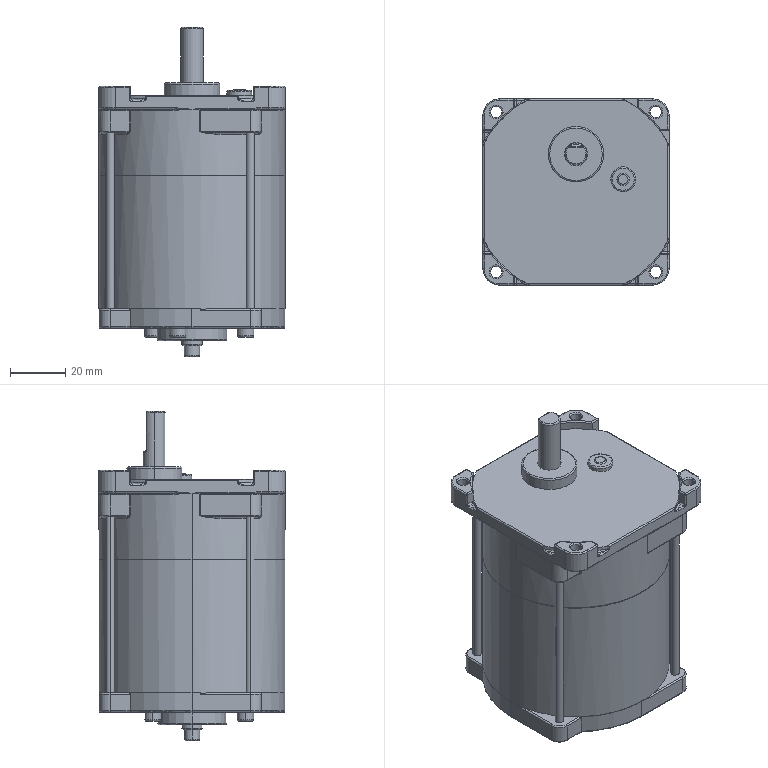Part | SolidWorks | features ICE 20, Fillet 6, Extrusion 1, RevCut 1 | 1 solid | 446 faces | box 67.25 x 67.25 x 118.75 mm | volume 309581 mm3 | cylinder 188 | torus 108 | plane 82 | spline 52 | sphere 16 | commonest cylinder face diameters 1 x100 3 x16 8 x12 75 x12 4 x8 2.75 x6